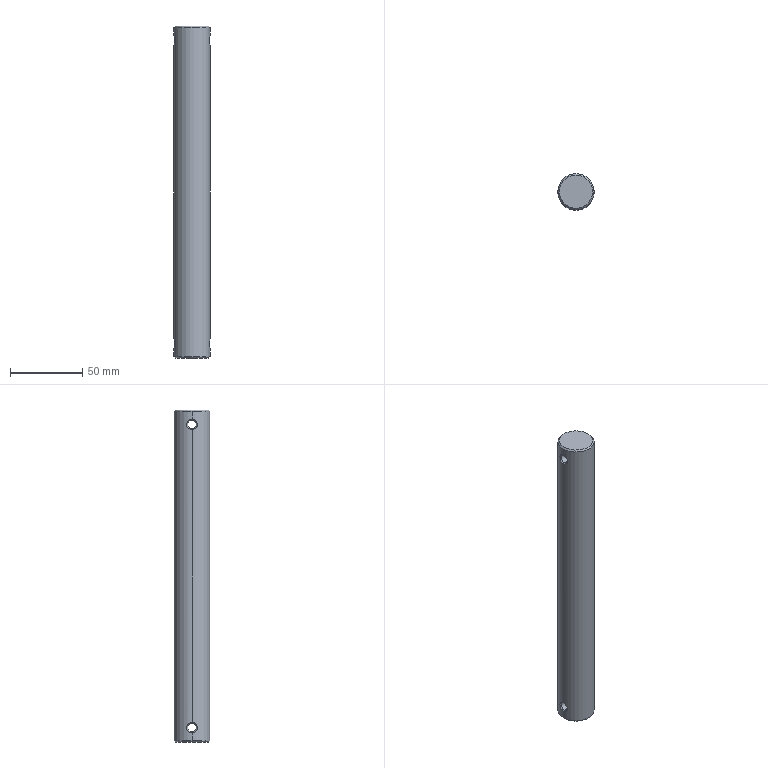Part | SolidWorks | features Chamfer 2, Extrusion 1, ICE 1 | 1 solid | 20 faces | box 25 x 25 x 230 mm | volume 111397 mm3 | spline 8 | cylinder 6 | cone 4 | plane 2 | commonest cylinder face diameters 6 x4 25 x2